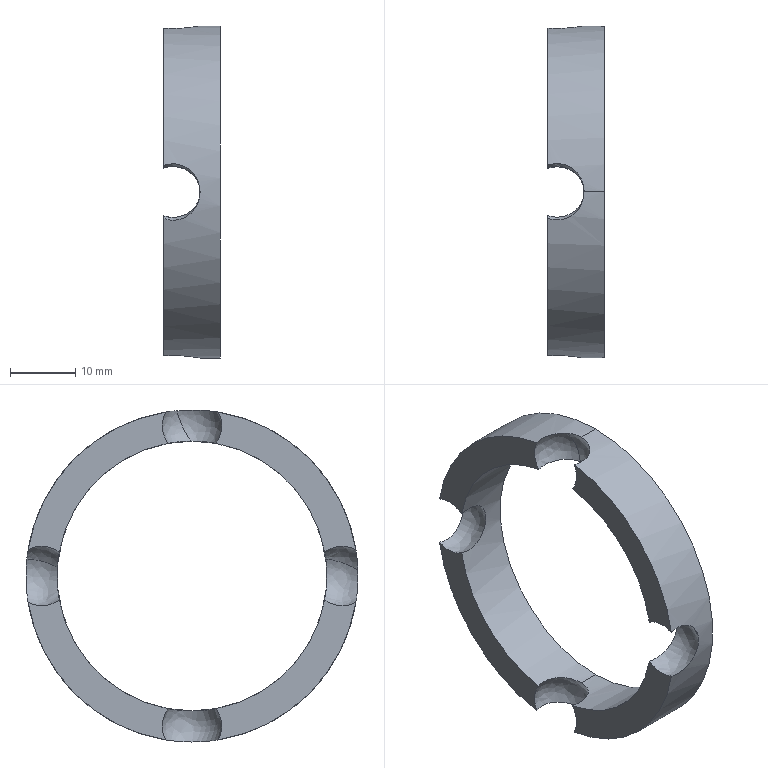Part | SolidWorks | features BaseBody 1 | 1 solid | 16 faces | box 8.629 x 50.763 x 50.763 mm | volume 5071 mm3 | spline 7 | plane 5 | cylinder 4 | commonest cylinder face diameters 41.237 x2 50.763 x2